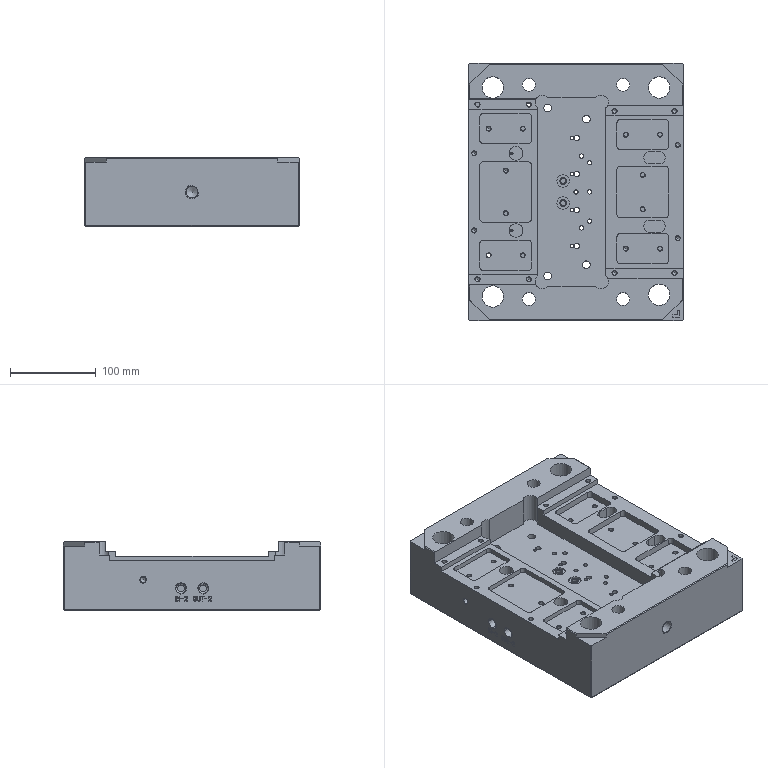NC program | PowerMill | posted with a generic post | part box 250 x 300 x 80 mm
Whole program:
%
O0001
N104 ( POWERMILL CB  : 2026004.0)
N105 ( POST VER      : 2026.0.0.5161)
N106 ( OPTION FILE   : FANUC)
N107 ( OUTPUT WORKPLANE : 1)
N108 (  )
N109 ( TOOL LIST )
N110 (----------------------------------------)
N111 ( NO. | ID         | DIA.| TIP RAD|LENGTH)
N112 (----------------------------------------)
N113 (    1|￠10中心钻_1|10.0 |  0.0   | 78.0 )
N114 (----------------------------------------)
N115 (  )
N116 ( NUMBER OF TOOLPATHS: 1.0 )
N117 ( ESTIMATED PROGRAM DURATION: 0 HOURS 1 MIN 18 SEC)
N118 (  )
N119 G00 G21 G80 G40 G17
N120 G90
N121 G54
N122 G53 Z0.0
N123 (---------------)
N124 ( START TOOLPATH : 01开粗-￠10中心钻-打中心点 )
N125 (---------------)
N126 ( TOOL NO.    :1 )
N127 ( TOOL TYPE   : DRILL)
N128 ( TOOL ID     : ￠10中心钻_1)
N129 ( TOOL DIA    : 10.0 LENGTH 78.0)
N130 T1
N131 M6
N132 S3000 M03
N133 G00 G90 X-21.0 Y-1.0
N134 G43 Z20.0 H1
N135
N136 G05 P10000 R8
N137 Z2.0
N138 G01 Z-2.0 F60.0
N139 G00 Z20.0
N140 Y4.6
N141 Z2.0
N142 G01 Z-2.0
N143 G00 Z20.0
N144 X-63.0
N145 Z2.0
N146 G01 Z-2.0
N147 G00 Z20.0
N148 X-98.0 Y33.0
N149 Z2.0
N150 G01 Z-2.0
N151 G00 Z20.0
N152 X-85.0 Y-12.0
N153 Z2.0
N154 G01 Z-2.0
N155 G00 Z20.0
N156 X-63.0 Y-1.0
N157 Z2.0
N158 G01 Z-2.0
N159 G00 Z20.0
N160 X-42.0 Y-6.5
N161 Z2.0
N162 G01 Z-2.0
N163 G00 Z20.0
N164 X-34.0 Y-16.0
N165 Z2.0
N166 G01 Z-2.0
N167 G00 Z20.0
N168 X0.0
N169 Z2.0
N170 G01 Z-2.0
N171 G00 Z20.0
N172 Y0.0
N173 Z2.0
N174 G01 Z-2.0
N175 G00 Z20.0
N176 X21.0 Y4.6
N177 Z2.0
N178 G01 Z-2.0
N179 G00 Z20.0
N180 Y-1.0
N181 Z2.0
N182 G01 Z-2.0
N183 G00 Z20.0
N184 X34.0 Y-16.0
N185 Z2.0
N186 G01 Z-2.0
N187 G00 Z20.0
N188 X42.0 Y-6.5
N189 Z2.0
N190 G01 Z-2.0
N191 G00 Z20.0
N192 X63.0 Y4.6
N193 Z2.0
N194 G01 Z-2.0
N195 G00 Z20.0
N196 Y-1.0
N197 Z2.0
N198 G01 Z-2.0
N199 G00 Z20.0
N200 X85.0 Y-12.0
N201 Z2.0
N202 G01 Z-2.0
N203 G00 Z20.0
N204 X98.0 Y33.0
N205 Z2.0
N206 G01 Z-2.0
N207 G00 Z20.0
N208 G05 P0
N209 (---------------)
N210 ( END TOOLPATH : 01开粗-￠10中心钻-打中心点 )
N211 (---------------)
N212
N213 M05
N214 G53 Z0.0
N215 M30
%